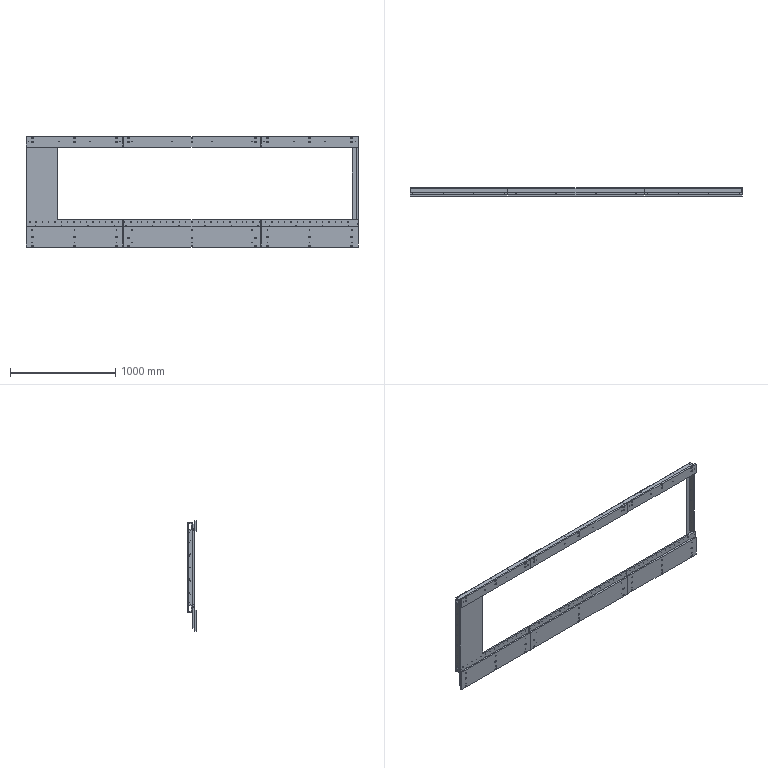Part | NX | features BREP 15 | 27 solids | 2204 faces | box 3152 x 78 x 1050 mm | volume 38052391 mm3 | cylinder 1310 | plane 694 | cone 200 | commonest cylinder face diameters 4.2 x512 10 x200 3.3 x176 15 x162 4.8 x80 6.8 x60